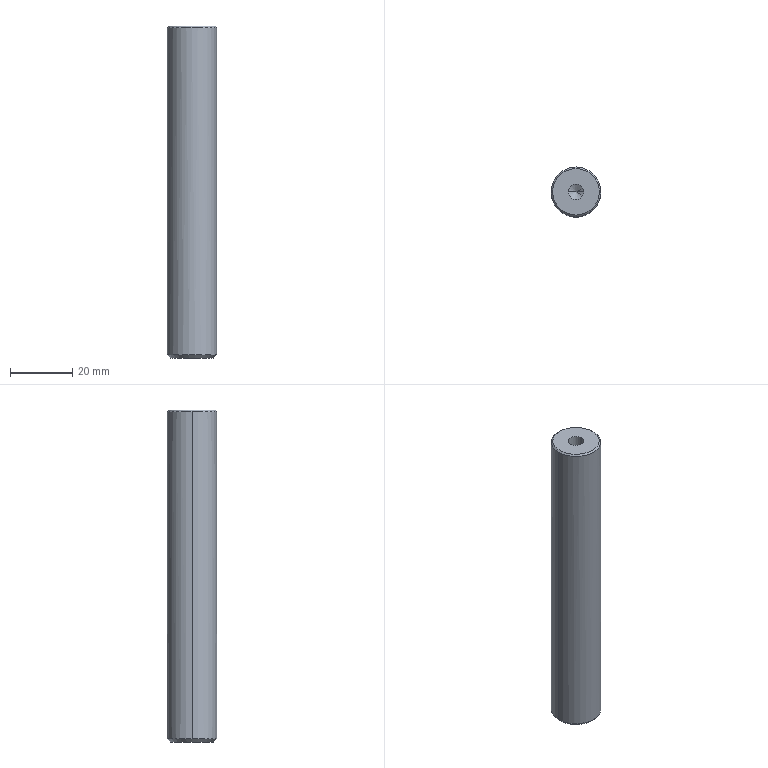Part | STEP file | PN_0006 Pre-compression sleeve guide rod | 1 solid | 16 faces | box 16 x 16 x 107 mm | volume 20796 mm3 | cone 8 | cylinder 6 | plane 2 | commonest cylinder face diameters 5 x4 16 x2
STEP:
#1=CARTESIAN_POINT('',(0.,0.,0.));
#2=DIRECTION('',(0.,0.,1.));
#3=DIRECTION('',(1.,0.,0.));
#4=AXIS2_PLACEMENT_3D('',#1,#2,#3);
#5=CARTESIAN_POINT('',(0.,8.,106.5));
#6=VERTEX_POINT('',#5);
#7=CARTESIAN_POINT('',(8.,0.,106.5));
#8=VERTEX_POINT('',#7);
#9=CARTESIAN_POINT('',(0.,0.,106.5));
#10=DIRECTION('',(0.,0.,-1.));
#11=DIRECTION('',(-1.,0.,0.));
#12=AXIS2_PLACEMENT_3D('',#9,#10,#11);
#13=CIRCLE('',#12,8.);
#14=CARTESIAN_POINT('',(0.,0.,107.));
#15=DIRECTION('',(0.,0.,-1.));
#16=DIRECTION('',(-1.,0.,0.));
#17=AXIS2_PLACEMENT_3D('',#14,#15,#16);
#18=CYLINDRICAL_SURFACE('',#17,8.);
#19=CARTESIAN_POINT('',(0.,0.5));
#20=DIRECTION('',(1.,0.));
#21=VECTOR('',#20,1.);
#22=LINE('',#19,#21);
#23=(GEOMETRIC_REPRESENTATION_CONTEXT(2)PARAMETRIC_REPRESENTATION_CONTEXT()REPRESENTATION_CONTEXT('',''));
#24=DEFINITIONAL_REPRESENTATION('',(#22),#23);
#25=PCURVE('',#18,#24);
#26=CARTESIAN_POINT('',(0.,0.,106.5));
#27=DIRECTION('',(0.,0.,-1.));
#28=DIRECTION('',(0.,1.,0.));
#29=AXIS2_PLACEMENT_3D('',#26,#27,#28);
#30=CONICAL_SURFACE('',#29,8.,0.7854);
#31=CARTESIAN_POINT('',(-1.571,0.));
#32=DIRECTION('',(1.,0.));
#33=VECTOR('',#32,1.);
#34=LINE('',#31,#33);
#35=(GEOMETRIC_REPRESENTATION_CONTEXT(2)PARAMETRIC_REPRESENTATION_CONTEXT()REPRESENTATION_CONTEXT('',''));
#36=DEFINITIONAL_REPRESENTATION('',(#34),#35);
#37=PCURVE('',#30,#36);
#38=SURFACE_CURVE('',#13,(#25,#37),.PCURVE_S1.);
#39=EDGE_CURVE('',#6,#8,#38,.T.);
#40=ORIENTED_EDGE('',*,*,#39,.T.);
#41=CARTESIAN_POINT('',(8.,0.,1.));
#42=VERTEX_POINT('',#41);
#43=CARTESIAN_POINT('',(8.,0.,107.));
#44=DIRECTION('',(0.,0.,-1.));
#45=VECTOR('',#44,1.);
#46=LINE('',#43,#45);
#47=CARTESIAN_POINT('',(3.142,0.));
#48=DIRECTION('',(0.,1.));
#49=VECTOR('',#48,1.);
#50=LINE('',#47,#49);
#51=(GEOMETRIC_REPRESENTATION_CONTEXT(2)PARAMETRIC_REPRESENTATION_CONTEXT()REPRESENTATION_CONTEXT('',''));
#52=DEFINITIONAL_REPRESENTATION('',(#50),#51);
#53=PCURVE('',#18,#52);
#54=CARTESIAN_POINT('',(0.,0.,107.));
#55=DIRECTION('',(0.,0.,-1.));
#56=DIRECTION('',(-1.,0.,0.));
#57=AXIS2_PLACEMENT_3D('',#54,#55,#56);
#58=CYLINDRICAL_SURFACE('',#57,8.);
#59=CARTESIAN_POINT('',(3.142,0.));
#60=DIRECTION('',(0.,1.));
#61=VECTOR('',#60,1.);
#62=LINE('',#59,#61);
#63=(GEOMETRIC_REPRESENTATION_CONTEXT(2)PARAMETRIC_REPRESENTATION_CONTEXT()REPRESENTATION_CONTEXT('',''));
#64=DEFINITIONAL_REPRESENTATION('',(#62),#63);
#65=PCURVE('',#58,#64);
#66=SURFACE_CURVE('',#46,(#53,#65),.PCURVE_S1.);
#67=EDGE_CURVE('',#8,#42,#66,.T.);
#68=ORIENTED_EDGE('',*,*,#67,.T.);
#69=CARTESIAN_POINT('',(-8.,0.,1.));
#70=VERTEX_POINT('',#69);
#71=CARTESIAN_POINT('',(0.,0.,1.));
#72=DIRECTION('',(0.,0.,1.));
#73=DIRECTION('',(-1.,0.,0.));
#74=AXIS2_PLACEMENT_3D('',#71,#72,#73);
#75=CIRCLE('',#74,8.);
#76=CARTESIAN_POINT('',(6.283,106.));
#77=DIRECTION('',(-1.,0.));
#78=VECTOR('',#77,1.);
#79=LINE('',#76,#78);
#80=(GEOMETRIC_REPRESENTATION_CONTEXT(2)PARAMETRIC_REPRESENTATION_CONTEXT()REPRESENTATION_CONTEXT('',''));
#81=DEFINITIONAL_REPRESENTATION('',(#79),#80);
#82=PCURVE('',#18,#81);
#83=CARTESIAN_POINT('',(0.,0.,1.));
#84=DIRECTION('',(0.,0.,1.));
#85=DIRECTION('',(1.,0.,0.));
#86=AXIS2_PLACEMENT_3D('',#83,#84,#85);
#87=CONICAL_SURFACE('',#86,8.,0.7854);
#88=CARTESIAN_POINT('',(-3.142,0.));
#89=DIRECTION('',(1.,0.));
#90=VECTOR('',#89,1.);
#91=LINE('',#88,#90);
#92=(GEOMETRIC_REPRESENTATION_CONTEXT(2)PARAMETRIC_REPRESENTATION_CONTEXT()REPRESENTATION_CONTEXT('',''));
#93=DEFINITIONAL_REPRESENTATION('',(#91),#92);
#94=PCURVE('',#87,#93);
#95=SURFACE_CURVE('',#75,(#82,#94),.PCURVE_S1.);
#96=EDGE_CURVE('',#42,#70,#95,.T.);
#97=ORIENTED_EDGE('',*,*,#96,.T.);
#98=CARTESIAN_POINT('',(-8.,0.,106.5));
#99=VERTEX_POINT('',#98);
#100=CARTESIAN_POINT('',(-8.,0.,107.));
#101=DIRECTION('',(0.,0.,-1.));
#102=VECTOR('',#101,1.);
#103=LINE('',#100,#102);
#104=CARTESIAN_POINT('',(0.,0.));
#105=DIRECTION('',(0.,1.));
#106=VECTOR('',#105,1.);
#107=LINE('',#104,#106);
#108=(GEOMETRIC_REPRESENTATION_CONTEXT(2)PARAMETRIC_REPRESENTATION_CONTEXT()REPRESENTATION_CONTEXT('',''));
#109=DEFINITIONAL_REPRESENTATION('',(#107),#108);
#110=PCURVE('',#18,#109);
#111=CARTESIAN_POINT('',(6.283,0.));
#112=DIRECTION('',(0.,1.));
#113=VECTOR('',#112,1.);
#114=LINE('',#111,#113);
#115=(GEOMETRIC_REPRESENTATION_CONTEXT(2)PARAMETRIC_REPRESENTATION_CONTEXT()REPRESENTATION_CONTEXT('',''));
#116=DEFINITIONAL_REPRESENTATION('',(#114),#115);
#117=PCURVE('',#58,#116);
#118=SURFACE_CURVE('',#103,(#110,#117),.PCURVE_S1.);
#119=EDGE_CURVE('',#99,#70,#118,.T.);
#120=ORIENTED_EDGE('',*,*,#119,.F.);
#121=CARTESIAN_POINT('',(0.,0.,106.5));
#122=DIRECTION('',(0.,0.,-1.));
#123=DIRECTION('',(-1.,0.,0.));
#124=AXIS2_PLACEMENT_3D('',#121,#122,#123);
#125=CIRCLE('',#124,8.);
#126=CARTESIAN_POINT('',(0.,0.5));
#127=DIRECTION('',(1.,0.));
#128=VECTOR('',#127,1.);
#129=LINE('',#126,#128);
#130=(GEOMETRIC_REPRESENTATION_CONTEXT(2)PARAMETRIC_REPRESENTATION_CONTEXT()REPRESENTATION_CONTEXT('',''));
#131=DEFINITIONAL_REPRESENTATION('',(#129),#130);
#132=PCURVE('',#18,#131);
#133=CARTESIAN_POINT('',(0.,0.,106.5));
#134=DIRECTION('',(0.,0.,-1.));
#135=DIRECTION('',(0.,1.,0.));
#136=AXIS2_PLACEMENT_3D('',#133,#134,#135);
#137=CONICAL_SURFACE('',#136,8.,0.7854);
#138=CARTESIAN_POINT('',(4.712,0.));
#139=DIRECTION('',(1.,0.));
#140=VECTOR('',#139,1.);
#141=LINE('',#138,#140);
#142=(GEOMETRIC_REPRESENTATION_CONTEXT(2)PARAMETRIC_REPRESENTATION_CONTEXT()REPRESENTATION_CONTEXT('',''));
#143=DEFINITIONAL_REPRESENTATION('',(#141),#142);
#144=PCURVE('',#137,#143);
#145=SURFACE_CURVE('',#125,(#132,#144),.PCURVE_S1.);
#146=EDGE_CURVE('',#99,#6,#145,.T.);
#147=ORIENTED_EDGE('',*,*,#146,.T.);
#148=EDGE_LOOP('',(#40,#68,#97,#120,#147));
#149=FACE_BOUND('',#148,.T.);
#150=ADVANCED_FACE('',(#149),#18,.T.);
#151=CARTESIAN_POINT('',(7.,0.,0.));
#152=VERTEX_POINT('',#151);
#153=CARTESIAN_POINT('',(-7.,0.,0.));
#154=VERTEX_POINT('',#153);
#155=CARTESIAN_POINT('',(0.,0.,0.));
#156=DIRECTION('',(0.,0.,1.));
#157=DIRECTION('',(1.,0.,0.));
#158=AXIS2_PLACEMENT_3D('',#155,#156,#157);
#159=CIRCLE('',#158,7.);
#160=CARTESIAN_POINT('',(0.,-1.));
#161=DIRECTION('',(1.,0.));
#162=VECTOR('',#161,1.);
#163=LINE('',#160,#162);
#164=(GEOMETRIC_REPRESENTATION_CONTEXT(2)PARAMETRIC_REPRESENTATION_CONTEXT()REPRESENTATION_CONTEXT('',''));
#165=DEFINITIONAL_REPRESENTATION('',(#163),#164);
#166=PCURVE('',#87,#165);
#167=CARTESIAN_POINT('',(0.,0.,0.));
#168=DIRECTION('',(0.,0.,1.));
#169=DIRECTION('',(1.,0.,0.));
#170=AXIS2_PLACEMENT_3D('',#167,#168,#169);
#171=PLANE('',#170);
#172=CARTESIAN_POINT('',(0.,0.));
#173=DIRECTION('',(1.,0.));
#174=AXIS2_PLACEMENT_2D('',#172,#173);
#175=CIRCLE('',#174,7.);
#176=(GEOMETRIC_REPRESENTATION_CONTEXT(2)PARAMETRIC_REPRESENTATION_CONTEXT()REPRESENTATION_CONTEXT('',''));
#177=DEFINITIONAL_REPRESENTATION('',(#175),#176);
#178=PCURVE('',#171,#177);
#179=SURFACE_CURVE('',#159,(#166,#178),.PCURVE_S1.);
#180=EDGE_CURVE('',#152,#154,#179,.T.);
#181=ORIENTED_EDGE('',*,*,#180,.T.);
#182=CARTESIAN_POINT('',(-8.,0.,1.));
#183=DIRECTION('',(-0.7071,0.,0.7071));
#184=VECTOR('',#183,1.);
#185=LINE('',#182,#184);
#186=CARTESIAN_POINT('',(3.142,0.));
#187=DIRECTION('',(0.,1.));
#188=VECTOR('',#187,1.);
#189=LINE('',#186,#188);
#190=(GEOMETRIC_REPRESENTATION_CONTEXT(2)PARAMETRIC_REPRESENTATION_CONTEXT()REPRESENTATION_CONTEXT('',''));
#191=DEFINITIONAL_REPRESENTATION('',(#189),#190);
#192=PCURVE('',#87,#191);
#193=CARTESIAN_POINT('',(0.,0.,1.));
#194=DIRECTION('',(0.,0.,1.));
#195=DIRECTION('',(1.,0.,0.));
#196=AXIS2_PLACEMENT_3D('',#193,#194,#195);
#197=CONICAL_SURFACE('',#196,8.,0.7854);
#198=CARTESIAN_POINT('',(3.142,0.));
#199=DIRECTION('',(0.,1.));
#200=VECTOR('',#199,1.);
#201=LINE('',#198,#200);
#202=(GEOMETRIC_REPRESENTATION_CONTEXT(2)PARAMETRIC_REPRESENTATION_CONTEXT()REPRESENTATION_CONTEXT('',''));
#203=DEFINITIONAL_REPRESENTATION('',(#201),#202);
#204=PCURVE('',#197,#203);
#205=SURFACE_CURVE('',#185,(#192,#204),.PCURVE_S1.);
#206=EDGE_CURVE('',#154,#70,#205,.T.);
#207=ORIENTED_EDGE('',*,*,#206,.T.);
#208=ORIENTED_EDGE('',*,*,#96,.F.);
#209=CARTESIAN_POINT('',(8.,0.,1.));
#210=DIRECTION('',(0.7071,0.,0.7071));
#211=VECTOR('',#210,1.);
#212=LINE('',#209,#211);
#213=CARTESIAN_POINT('',(0.,0.));
#214=DIRECTION('',(0.,1.));
#215=VECTOR('',#214,1.);
#216=LINE('',#213,#215);
#217=(GEOMETRIC_REPRESENTATION_CONTEXT(2)PARAMETRIC_REPRESENTATION_CONTEXT()REPRESENTATION_CONTEXT('',''));
#218=DEFINITIONAL_REPRESENTATION('',(#216),#217);
#219=PCURVE('',#87,#218);
#220=CARTESIAN_POINT('',(6.283,0.));
#221=DIRECTION('',(0.,1.));
#222=VECTOR('',#221,1.);
#223=LINE('',#220,#222);
#224=(GEOMETRIC_REPRESENTATION_CONTEXT(2)PARAMETRIC_REPRESENTATION_CONTEXT()REPRESENTATION_CONTEXT('',''));
#225=DEFINITIONAL_REPRESENTATION('',(#223),#224);
#226=PCURVE('',#197,#225);
#227=SURFACE_CURVE('',#212,(#219,#226),.PCURVE_S1.);
#228=EDGE_CURVE('',#152,#42,#227,.T.);
#229=ORIENTED_EDGE('',*,*,#228,.F.);
#230=EDGE_LOOP('',(#181,#207,#208,#229));
#231=FACE_BOUND('',#230,.T.);
#232=ADVANCED_FACE('',(#231),#87,.T.);
#233=CARTESIAN_POINT('',(0.,7.5,107.));
#234=VERTEX_POINT('',#233);
#235=CARTESIAN_POINT('',(0.,-7.5,107.));
#236=VERTEX_POINT('',#235);
#237=CARTESIAN_POINT('',(0.,0.,107.));
#238=DIRECTION('',(0.,0.,-1.));
#239=DIRECTION('',(0.,1.,0.));
#240=AXIS2_PLACEMENT_3D('',#237,#238,#239);
#241=CIRCLE('',#240,7.5);
#242=CARTESIAN_POINT('',(0.,-0.5));
#243=DIRECTION('',(1.,0.));
#244=VECTOR('',#243,1.);
#245=LINE('',#242,#244);
#246=(GEOMETRIC_REPRESENTATION_CONTEXT(2)PARAMETRIC_REPRESENTATION_CONTEXT()REPRESENTATION_CONTEXT('',''));
#247=DEFINITIONAL_REPRESENTATION('',(#245),#246);
#248=PCURVE('',#30,#247);
#249=CARTESIAN_POINT('',(0.,0.,107.));
#250=DIRECTION('',(0.,0.,1.));
#251=DIRECTION('',(1.,0.,0.));
#252=AXIS2_PLACEMENT_3D('',#249,#250,#251);
#253=PLANE('',#252);
#254=CARTESIAN_POINT('',(0.,7.5));
#255=CARTESIAN_POINT('',(12.99,7.5));
#256=CARTESIAN_POINT('',(6.495,-3.75));
#257=CARTESIAN_POINT('',(0.,-15.));
#258=CARTESIAN_POINT('',(-6.495,-3.75));
#259=CARTESIAN_POINT('',(-12.99,7.5));
#260=CARTESIAN_POINT('',(0.,7.5));
#261=(BOUNDED_CURVE()B_SPLINE_CURVE(2,(#254,#255,#256,#257,#258,#259,#260),.UNSPECIFIED.,.T.,.F.)B_SPLINE_CURVE_WITH_KNOTS((1,2,2,2,2,1),(-2.094,0.,2.094,4.189,6.283,8.378),.UNSPECIFIED.)CURVE()GEOMETRIC_REPRESENTATION_ITEM()RATIONAL_B_SPLINE_CURVE((1.,0.5,1.,0.5,1.,0.5,1.))REPRESENTATION_ITEM(''));
#262=(GEOMETRIC_REPRESENTATION_CONTEXT(2)PARAMETRIC_REPRESENTATION_CONTEXT()REPRESENTATION_CONTEXT('',''));
#263=DEFINITIONAL_REPRESENTATION('',(#261),#262);
#264=PCURVE('',#253,#263);
#265=SURFACE_CURVE('',#241,(#248,#264),.PCURVE_S1.);
#266=EDGE_CURVE('',#234,#236,#265,.T.);
#267=ORIENTED_EDGE('',*,*,#266,.T.);
#268=CARTESIAN_POINT('',(0.,-8.,106.5));
#269=VERTEX_POINT('',#268);
#270=CARTESIAN_POINT('',(0.,-8.,106.5));
#271=DIRECTION('',(0.,-0.7071,-0.7071));
#272=VECTOR('',#271,1.);
#273=LINE('',#270,#272);
#274=CARTESIAN_POINT('',(3.142,0.));
#275=DIRECTION('',(0.,1.));
#276=VECTOR('',#275,1.);
#277=LINE('',#274,#276);
#278=(GEOMETRIC_REPRESENTATION_CONTEXT(2)PARAMETRIC_REPRESENTATION_CONTEXT()REPRESENTATION_CONTEXT('',''));
#279=DEFINITIONAL_REPRESENTATION('',(#277),#278);
#280=PCURVE('',#30,#279);
#281=CARTESIAN_POINT('',(3.142,0.));
#282=DIRECTION('',(0.,1.));
#283=VECTOR('',#282,1.);
#284=LINE('',#281,#283);
#285=(GEOMETRIC_REPRESENTATION_CONTEXT(2)PARAMETRIC_REPRESENTATION_CONTEXT()REPRESENTATION_CONTEXT('',''));
#286=DEFINITIONAL_REPRESENTATION('',(#284),#285);
#287=PCURVE('',#137,#286);
#288=SURFACE_CURVE('',#273,(#280,#287),.PCURVE_S1.);
#289=EDGE_CURVE('',#236,#269,#288,.T.);
#290=ORIENTED_EDGE('',*,*,#289,.T.);
#291=CARTESIAN_POINT('',(0.,0.,106.5));
#292=DIRECTION('',(0.,0.,-1.));
#293=DIRECTION('',(-1.,0.,0.));
#294=AXIS2_PLACEMENT_3D('',#291,#292,#293);
#295=CIRCLE('',#294,8.);
#296=CARTESIAN_POINT('',(-1.571,0.));
#297=DIRECTION('',(1.,0.));
#298=VECTOR('',#297,1.);
#299=LINE('',#296,#298);
#300=(GEOMETRIC_REPRESENTATION_CONTEXT(2)PARAMETRIC_REPRESENTATION_CONTEXT()REPRESENTATION_CONTEXT('',''));
#301=DEFINITIONAL_REPRESENTATION('',(#299),#300);
#302=PCURVE('',#30,#301);
#303=CARTESIAN_POINT('',(0.,0.5));
#304=DIRECTION('',(1.,0.));
#305=VECTOR('',#304,1.);
#306=LINE('',#303,#305);
#307=(GEOMETRIC_REPRESENTATION_CONTEXT(2)PARAMETRIC_REPRESENTATION_CONTEXT()REPRESENTATION_CONTEXT('',''));
#308=DEFINITIONAL_REPRESENTATION('',(#306),#307);
#309=PCURVE('',#58,#308);
#310=SURFACE_CURVE('',#295,(#302,#309),.PCURVE_S1.);
#311=EDGE_CURVE('',#8,#269,#310,.T.);
#312=ORIENTED_EDGE('',*,*,#311,.F.);
#313=ORIENTED_EDGE('',*,*,#39,.F.);
#314=CARTESIAN_POINT('',(0.,8.,106.5));
#315=DIRECTION('',(0.,0.7071,-0.7071));
#316=VECTOR('',#315,1.);
#317=LINE('',#314,#316);
#318=CARTESIAN_POINT('',(0.,0.));
#319=DIRECTION('',(0.,1.));
#320=VECTOR('',#319,1.);
#321=LINE('',#318,#320);
#322=(GEOMETRIC_REPRESENTATION_CONTEXT(2)PARAMETRIC_REPRESENTATION_CONTEXT()REPRESENTATION_CONTEXT('',''));
#323=DEFINITIONAL_REPRESENTATION('',(#321),#322);
#324=PCURVE('',#30,#323);
#325=CARTESIAN_POINT('',(6.283,0.));
#326=DIRECTION('',(0.,1.));
#327=VECTOR('',#326,1.);
#328=LINE('',#325,#327);
#329=(GEOMETRIC_REPRESENTATION_CONTEXT(2)PARAMETRIC_REPRESENTATION_CONTEXT()REPRESENTATION_CONTEXT('',''));
#330=DEFINITIONAL_REPRESENTATION('',(#328),#329);
#331=PCURVE('',#137,#330);
#332=SURFACE_CURVE('',#317,(#324,#331),.PCURVE_S1.);
#333=EDGE_CURVE('',#234,#6,#332,.T.);
#334=ORIENTED_EDGE('',*,*,#333,.F.);
#335=EDGE_LOOP('',(#267,#290,#312,#313,#334));
#336=FACE_BOUND('',#335,.T.);
#337=ADVANCED_FACE('',(#336),#30,.T.);
#338=CARTESIAN_POINT('',(-2.5,0.,17.));
#339=VERTEX_POINT('',#338);
#340=CARTESIAN_POINT('',(-2.5,0.,0.));
#341=VERTEX_POINT('',#340);
#342=CARTESIAN_POINT('',(-2.5,0.,0.));
#343=DIRECTION('',(0.,0.,-1.));
#344=VECTOR('',#343,1.);
#345=LINE('',#342,#344);
#346=CARTESIAN_POINT('',(0.,0.,0.));
#347=DIRECTION('',(0.,0.,-1.));
#348=DIRECTION('',(-1.,0.,0.));
#349=AXIS2_PLACEMENT_3D('',#346,#347,#348);
#350=CYLINDRICAL_SURFACE('',#349,2.5);
#351=CARTESIAN_POINT('',(6.283,0.));
#352=DIRECTION('',(0.,1.));
#353=VECTOR('',#352,1.);
#354=LINE('',#351,#353);
#355=(GEOMETRIC_REPRESENTATION_CONTEXT(2)PARAMETRIC_REPRESENTATION_CONTEXT()REPRESENTATION_CONTEXT('',''));
#356=DEFINITIONAL_REPRESENTATION('',(#354),#355);
#357=PCURVE('',#350,#356);
#358=CARTESIAN_POINT('',(0.,0.,0.));
#359=DIRECTION('',(0.,0.,-1.));
#360=DIRECTION('',(-1.,0.,0.));
#361=AXIS2_PLACEMENT_3D('',#358,#359,#360);
#362=CYLINDRICAL_SURFACE('',#361,2.5);
#363=CARTESIAN_POINT('',(0.,0.));
#364=DIRECTION('',(0.,1.));
#365=VECTOR('',#364,1.);
#366=LINE('',#363,#365);
#367=(GEOMETRIC_REPRESENTATION_CONTEXT(2)PARAMETRIC_REPRESENTATION_CONTEXT()REPRESENTATION_CONTEXT('',''));
#368=DEFINITIONAL_REPRESENTATION('',(#366),#367);
#369=PCURVE('',#362,#368);
#370=SURFACE_CURVE('',#345,(#357,#369),.PCURVE_S1.);
#371=EDGE_CURVE('',#339,#341,#370,.T.);
#372=ORIENTED_EDGE('',*,*,#371,.T.);
#373=CARTESIAN_POINT('',(2.5,0.,0.));
#374=VERTEX_POINT('',#373);
#375=CARTESIAN_POINT('',(0.,0.,0.));
#376=DIRECTION('',(0.,0.,-1.));
#377=DIRECTION('',(-1.,0.,0.));
#378=AXIS2_PLACEMENT_3D('',#375,#376,#377);
#379=CIRCLE('',#378,2.5);
#380=CARTESIAN_POINT('',(0.,0.));
#381=DIRECTION('',(1.,0.));
#382=VECTOR('',#381,1.);
#383=LINE('',#380,#382);
#384=(GEOMETRIC_REPRESENTATION_CONTEXT(2)PARAMETRIC_REPRESENTATION_CONTEXT()REPRESENTATION_CONTEXT('',''));
#385=DEFINITIONAL_REPRESENTATION('',(#383),#384);
#386=PCURVE('',#350,#385);
#387=CARTESIAN_POINT('',(-2.5,0.));
#388=CARTESIAN_POINT('',(-2.5,4.33));
#389=CARTESIAN_POINT('',(1.25,2.165));
#390=CARTESIAN_POINT('',(5.,0.));
#391=CARTESIAN_POINT('',(1.25,-2.165));
#392=CARTESIAN_POINT('',(-2.5,-4.33));
#393=CARTESIAN_POINT('',(-2.5,0.));
#394=(BOUNDED_CURVE()B_SPLINE_CURVE(2,(#387,#388,#389,#390,#391,#392,#393),.UNSPECIFIED.,.T.,.F.)B_SPLINE_CURVE_WITH_KNOTS((1,2,2,2,2,1),(-2.094,0.,2.094,4.189,6.283,8.378),.UNSPECIFIED.)CURVE()GEOMETRIC_REPRESENTATION_ITEM()RATIONAL_B_SPLINE_CURVE((1.,0.5,1.,0.5,1.,0.5,1.))REPRESENTATION_ITEM(''));
#395=(GEOMETRIC_REPRESENTATION_CONTEXT(2)PARAMETRIC_REPRESENTATION_CONTEXT()REPRESENTATION_CONTEXT('',''));
#396=DEFINITIONAL_REPRESENTATION('',(#394),#395);
#397=PCURVE('',#171,#396);
#398=SURFACE_CURVE('',#379,(#386,#397),.PCURVE_S1.);
#399=EDGE_CURVE('',#374,#341,#398,.T.);
#400=ORIENTED_EDGE('',*,*,#399,.F.);
#401=CARTESIAN_POINT('',(2.5,0.,17.));
#402=VERTEX_POINT('',#401);
#403=CARTESIAN_POINT('',(2.5,0.,0.));
#404=DIRECTION('',(0.,0.,-1.));
#405=VECTOR('',#404,1.);
#406=LINE('',#403,#405);
#407=CARTESIAN_POINT('',(3.142,0.));
#408=DIRECTION('',(0.,1.));
#409=VECTOR('',#408,1.);
#410=LINE('',#407,#409);
#411=(GEOMETRIC_REPRESENTATION_CONTEXT(2)PARAMETRIC_REPRESENTATION_CONTEXT()REPRESENTATION_CONTEXT('',''));
#412=DEFINITIONAL_REPRESENTATION('',(#410),#411);
#413=PCURVE('',#350,#412);
#414=CARTESIAN_POINT('',(3.142,0.));
#415=DIRECTION('',(0.,1.));
#416=VECTOR('',#415,1.);
#417=LINE('',#414,#416);
#418=(GEOMETRIC_REPRESENTATION_CONTEXT(2)PARAMETRIC_REPRESENTATION_CONTEXT()REPRESENTATION_CONTEXT('',''));
#419=DEFINITIONAL_REPRESENTATION('',(#417),#418);
#420=PCURVE('',#362,#419);
#421=SURFACE_CURVE('',#406,(#413,#420),.PCURVE_S1.);
#422=EDGE_CURVE('',#402,#374,#421,.T.);
#423=ORIENTED_EDGE('',*,*,#422,.F.);
#424=CARTESIAN_POINT('',(0.,0.,17.));
#425=DIRECTION('',(0.,0.,-1.));
#426=DIRECTION('',(-1.,0.,0.));
#427=AXIS2_PLACEMENT_3D('',#424,#425,#426);
#428=CIRCLE('',#427,2.5);
#429=CARTESIAN_POINT('',(0.,-17.));
#430=DIRECTION('',(1.,0.));
#431=VECTOR('',#430,1.);
#432=LINE('',#429,#431);
#433=(GEOMETRIC_REPRESENTATION_CONTEXT(2)PARAMETRIC_REPRESENTATION_CONTEXT()REPRESENTATION_CONTEXT('',''));
#434=DEFINITIONAL_REPRESENTATION('',(#432),#433);
#435=PCURVE('',#350,#434);
#436=CARTESIAN_POINT('',(0.,0.,17.));
#437=DIRECTION('',(0.,0.,-1.));
#438=DIRECTION('',(-1.,0.,0.));
#439=AXIS2_PLACEMENT_3D('',#436,#437,#438);
#440=CONICAL_SURFACE('',#439,2.5,1.03);
#441=CARTESIAN_POINT('',(0.,0.));
#442=DIRECTION('',(1.,0.));
#443=VECTOR('',#442,1.);
#444=LINE('',#441,#443);
#445=(GEOMETRIC_REPRESENTATION_CONTEXT(2)PARAMETRIC_REPRESENTATION_CONTEXT()REPRESENTATION_CONTEXT('',''));
#446=DEFINITIONAL_REPRESENTATION('',(#444),#445);
#447=PCURVE('',#440,#446);
#448=SURFACE_CURVE('',#428,(#435,#447),.PCURVE_S1.);
#449=EDGE_CURVE('',#402,#339,#448,.T.);
#450=ORIENTED_EDGE('',*,*,#449,.T.);
#451=EDGE_LOOP('',(#372,#400,#423,#450));
#452=FACE_BOUND('',#451,.F.);
#453=ADVANCED_FACE('',(#452),#350,.F.);
#454=CARTESIAN_POINT('',(2.5,0.,90.));
#455=VERTEX_POINT('',#454);
#456=CARTESIAN_POINT('',(2.5,0.,107.));
#457=VERTEX_POINT('',#456);
#458=CARTESIAN_POINT('',(2.5,0.,107.));
#459=DIRECTION('',(0.,0.,1.));
#460=VECTOR('',#459,1.);
#461=LINE('',#458,#460);
#462=CARTESIAN_POINT('',(0.,0.,107.));
#463=DIRECTION('',(0.,0.,1.));
#464=DIRECTION('',(1.,0.,0.));
#465=AXIS2_PLACEMENT_3D('',#462,#463,#464);
#466=CYLINDRICAL_SURFACE('',#465,2.5);
#467=CARTESIAN_POINT('',(6.283,0.));
#468=DIRECTION('',(0.,1.));
#469=VECTOR('',#468,1.);
#470=LINE('',#467,#469);
#471=(GEOMETRIC_REPRESENTATION_CONTEXT(2)PARAMETRIC_REPRESENTATION_CONTEXT()REPRESENTATION_CONTEXT('',''));
#472=DEFINITIONAL_REPRESENTATION('',(#470),#471);
#473=PCURVE('',#466,#472);
#474=CARTESIAN_POINT('',(0.,0.,107.));
#475=DIRECTION('',(0.,0.,1.));
#476=DIRECTION('',(1.,0.,0.));
#477=AXIS2_PLACEMENT_3D('',#474,#475,#476);
#478=CYLINDRICAL_SURFACE('',#477,2.5);
#479=CARTESIAN_POINT('',(0.,0.));
#480=DIRECTION('',(0.,1.));
#481=VECTOR('',#480,1.);
#482=LINE('',#479,#481);
#483=(GEOMETRIC_REPRESENTATION_CONTEXT(2)PARAMETRIC_REPRESENTATION_CONTEXT()REPRESENTATION_CONTEXT('',''));
#484=DEFINITIONAL_REPRESENTATION('',(#482),#483);
#485=PCURVE('',#478,#484);
#486=SURFACE_CURVE('',#461,(#473,#485),.PCURVE_S1.);
#487=EDGE_CURVE('',#455,#457,#486,.T.);
#488=ORIENTED_EDGE('',*,*,#487,.T.);
#489=CARTESIAN_POINT('',(-2.5,0.,107.));
#490=VERTEX_POINT('',#489);
#491=CARTESIAN_POINT('',(0.,0.,107.));
#492=DIRECTION('',(0.,0.,-1.));
#493=DIRECTION('',(1.,0.,0.));
#494=AXIS2_PLACEMENT_3D('',#491,#492,#493);
#495=CIRCLE('',#494,2.5);
#496=CARTESIAN_POINT('',(6.283,0.));
#497=DIRECTION('',(-1.,0.));
#498=VECTOR('',#497,1.);
#499=LINE('',#496,#498);
#500=(GEOMETRIC_REPRESENTATION_CONTEXT(2)PARAMETRIC_REPRESENTATION_CONTEXT()REPRESENTATION_CONTEXT('',''));
#501=DEFINITIONAL_REPRESENTATION('',(#499),#500);
#502=PCURVE('',#466,#501);
#503=CARTESIAN_POINT('',(2.5,0.));
#504=CARTESIAN_POINT('',(2.5,-4.33));
#505=CARTESIAN_POINT('',(-1.25,-2.165));
#506=CARTESIAN_POINT('',(-5.,0.));
#507=CARTESIAN_POINT('',(-1.25,2.165));
#508=CARTESIAN_POINT('',(2.5,4.33));
#509=CARTESIAN_POINT('',(2.5,0.));
#510=(BOUNDED_CURVE()B_SPLINE_CURVE(2,(#503,#504,#505,#506,#507,#508,#509),.UNSPECIFIED.,.T.,.F.)B_SPLINE_CURVE_WITH_KNOTS((1,2,2,2,2,1),(-2.094,0.,2.094,4.189,6.283,8.378),.UNSPECIFIED.)CURVE()GEOMETRIC_REPRESENTATION_ITEM()RATIONAL_B_SPLINE_CURVE((1.,0.5,1.,0.5,1.,0.5,1.))REPRESENTATION_ITEM(''));
#511=(GEOMETRIC_REPRESENTATION_CONTEXT(2)PARAMETRIC_REPRESENTATION_CONTEXT()REPRESENTATION_CONTEXT('',''));
#512=DEFINITIONAL_REPRESENTATION('',(#510),#511);
#513=PCURVE('',#253,#512);
#514=SURFACE_CURVE('',#495,(#502,#513),.PCURVE_S1.);
#515=EDGE_CURVE('',#457,#490,#514,.T.);
#516=ORIENTED_EDGE('',*,*,#515,.T.);
#517=CARTESIAN_POINT('',(-2.5,0.,90.));
#518=VERTEX_POINT('',#517);
#519=CARTESIAN_POINT('',(-2.5,0.,107.));
#520=DIRECTION('',(0.,0.,1.));
#521=VECTOR('',#520,1.);
#522=LINE('',#519,#521);
#523=CARTESIAN_POINT('',(3.142,0.));
#524=DIRECTION('',(0.,1.));
#525=VECTOR('',#524,1.);
#526=LINE('',#523,#525);
#527=(GEOMETRIC_REPRESENTATION_CONTEXT(2)PARAMETRIC_REPRESENTATION_CONTEXT()REPRESENTATION_CONTEXT('',''));
#528=DEFINITIONAL_REPRESENTATION('',(#526),#527);
#529=PCURVE('',#466,#528);
#530=CARTESIAN_POINT('',(3.142,0.));
#531=DIRECTION('',(0.,1.));
#532=VECTOR('',#531,1.);
#533=LINE('',#530,#532);
#534=(GEOMETRIC_REPRESENTATION_CONTEXT(2)PARAMETRIC_REPRESENTATION_CONTEXT()REPRESENTATION_CONTEXT('',''));
#535=DEFINITIONAL_REPRESENTATION('',(#533),#534);
#536=PCURVE('',#478,#535);
#537=SURFACE_CURVE('',#522,(#529,#536),.PCURVE_S1.);
#538=EDGE_CURVE('',#518,#490,#537,.T.);
#539=ORIENTED_EDGE('',*,*,#538,.F.);
#540=CARTESIAN_POINT('',(0.,0.,90.));
#541=DIRECTION('',(0.,0.,1.));
#542=DIRECTION('',(1.,0.,0.));
#543=AXIS2_PLACEMENT_3D('',#540,#541,#542);
#544=CIRCLE('',#543,2.5);
#545=CARTESIAN_POINT('',(0.,-17.));
#546=DIRECTION('',(1.,0.));
#547=VECTOR('',#546,1.);
#548=LINE('',#545,#547);
#549=(GEOMETRIC_REPRESENTATION_CONTEXT(2)PARAMETRIC_REPRESENTATION_CONTEXT()REPRESENTATION_CONTEXT('',''));
#550=DEFINITIONAL_REPRESENTATION('',(#548),#549);
#551=PCURVE('',#466,#550);
#552=CARTESIAN_POINT('',(0.,0.,90.));
#553=DIRECTION('',(0.,0.,1.));
#554=DIRECTION('',(1.,0.,0.));
#555=AXIS2_PLACEMENT_3D('',#552,#553,#554);
#556=CONICAL_SURFACE('',#555,2.5,1.03);
#557=CARTESIAN_POINT('',(0.,0.));
#558=DIRECTION('',(1.,0.));
#559=VECTOR('',#558,1.);
#560=LINE('',#557,#559);
#561=(GEOMETRIC_REPRESENTATION_CONTEXT(2)PARAMETRIC_REPRESENTATION_CONTEXT()REPRESENTATION_CONTEXT('',''));
#562=DEFINITIONAL_REPRESENTATION('',(#560),#561);
#563=PCURVE('',#556,#562);
#564=SURFACE_CURVE('',#544,(#551,#563),.PCURVE_S1.);
#565=EDGE_CURVE('',#518,#455,#564,.T.);
#566=ORIENTED_EDGE('',*,*,#565,.T.);
#567=EDGE_LOOP('',(#488,#516,#539,#566));
#568=FACE_BOUND('',#567,.F.);
#569=ADVANCED_FACE('',(#568),#466,.F.);
#570=ORIENTED_EDGE('',*,*,#449,.F.);
#571=CARTESIAN_POINT('',(0.,0.,18.502));
#572=VERTEX_POINT('',#571);
#573=CARTESIAN_POINT('',(2.5,0.,17.));
#574=DIRECTION('',(0.8572,0.,-0.515));
#575=VECTOR('',#574,1.);
#576=LINE('',#573,#575);
#577=CARTESIAN_POINT('',(3.142,0.));
#578=DIRECTION('',(0.,1.));
#579=VECTOR('',#578,1.);
#580=LINE('',#577,#579);
#581=(GEOMETRIC_REPRESENTATION_CONTEXT(2)PARAMETRIC_REPRESENTATION_CONTEXT()REPRESENTATION_CONTEXT('',''));
#582=DEFINITIONAL_REPRESENTATION('',(#580),#581);
#583=PCURVE('',#440,#582);
#584=CARTESIAN_POINT('',(0.,0.,17.));
#585=DIRECTION('',(0.,0.,-1.));
#586=DIRECTION('',(-1.,0.,0.));
#587=AXIS2_PLACEMENT_3D('',#584,#585,#586);
#588=CONICAL_SURFACE('',#587,2.5,1.03);
#589=CARTESIAN_POINT('',(3.142,0.));
#590=DIRECTION('',(0.,1.));
#591=VECTOR('',#590,1.);
#592=LINE('',#589,#591);
#593=(GEOMETRIC_REPRESENTATION_CONTEXT(2)PARAMETRIC_REPRESENTATION_CONTEXT()REPRESENTATION_CONTEXT('',''));
#594=DEFINITIONAL_REPRESENTATION('',(#592),#593);
#595=PCURVE('',#588,#594);
#596=SURFACE_CURVE('',#576,(#583,#595),.PCURVE_S1.);
#597=EDGE_CURVE('',#572,#402,#596,.T.);
#598=ORIENTED_EDGE('',*,*,#597,.F.);
#599=CARTESIAN_POINT('',(-2.5,0.,17.));
#600=DIRECTION('',(-0.8572,0.,-0.515));
#601=VECTOR('',#600,1.);
#602=LINE('',#599,#601);
#603=CARTESIAN_POINT('',(6.283,0.));
#604=DIRECTION('',(0.,1.));
#605=VECTOR('',#604,1.);
#606=LINE('',#603,#605);
#607=(GEOMETRIC_REPRESENTATION_CONTEXT(2)PARAMETRIC_REPRESENTATION_CONTEXT()REPRESENTATION_CONTEXT('',''));
#608=DEFINITIONAL_REPRESENTATION('',(#606),#607);
#609=PCURVE('',#440,#608);
#610=CARTESIAN_POINT('',(0.,0.));
#611=DIRECTION('',(0.,1.));
#612=VECTOR('',#611,1.);
#613=LINE('',#610,#612);
#614=(GEOMETRIC_REPRESENTATION_CONTEXT(2)PARAMETRIC_REPRESENTATION_CONTEXT()REPRESENTATION_CONTEXT('',''));
#615=DEFINITIONAL_REPRESENTATION('',(#613),#614);
#616=PCURVE('',#588,#615);
#617=SURFACE_CURVE('',#602,(#609,#616),.PCURVE_S1.);
#618=EDGE_CURVE('',#572,#339,#617,.T.);
#619=ORIENTED_EDGE('',*,*,#618,.T.);
#620=EDGE_LOOP('',(#570,#598,#619));
#621=FACE_BOUND('',#620,.F.);
#622=ADVANCED_FACE('',(#621),#440,.F.);
#623=ORIENTED_EDGE('',*,*,#565,.F.);
#624=CARTESIAN_POINT('',(0.,0.,88.498));
#625=VERTEX_POINT('',#624);
#626=CARTESIAN_POINT('',(-2.5,0.,90.));
#627=DIRECTION('',(-0.8572,0.,0.515));
#628=VECTOR('',#627,1.);
#629=LINE('',#626,#628);
#630=CARTESIAN_POINT('',(3.142,0.));
#631=DIRECTION('',(0.,1.));
#632=VECTOR('',#631,1.);
#633=LINE('',#630,#632);
#634=(GEOMETRIC_REPRESENTATION_CONTEXT(2)PARAMETRIC_REPRESENTATION_CONTEXT()REPRESENTATION_CONTEXT('',''));
#635=DEFINITIONAL_REPRESENTATION('',(#633),#634);
#636=PCURVE('',#556,#635);
#637=CARTESIAN_POINT('',(0.,0.,90.));
#638=DIRECTION('',(0.,0.,1.));
#639=DIRECTION('',(1.,0.,0.));
#640=AXIS2_PLACEMENT_3D('',#637,#638,#639);
#641=CONICAL_SURFACE('',#640,2.5,1.03);
#642=CARTESIAN_POINT('',(3.142,0.));
#643=DIRECTION('',(0.,1.));
#644=VECTOR('',#643,1.);
#645=LINE('',#642,#644);
#646=(GEOMETRIC_REPRESENTATION_CONTEXT(2)PARAMETRIC_REPRESENTATION_CONTEXT()REPRESENTATION_CONTEXT('',''));
#647=DEFINITIONAL_REPRESENTATION('',(#645),#646);
#648=PCURVE('',#641,#647);
#649=SURFACE_CURVE('',#629,(#636,#648),.PCURVE_S1.);
#650=EDGE_CURVE('',#625,#518,#649,.T.);
#651=ORIENTED_EDGE('',*,*,#650,.F.);
#652=CARTESIAN_POINT('',(2.5,0.,90.));
#653=DIRECTION('',(0.8572,0.,0.515));
#654=VECTOR('',#653,1.);
#655=LINE('',#652,#654);
#656=CARTESIAN_POINT('',(6.283,0.));
#657=DIRECTION('',(0.,1.));
#658=VECTOR('',#657,1.);
#659=LINE('',#656,#658);
#660=(GEOMETRIC_REPRESENTATION_CONTEXT(2)PARAMETRIC_REPRESENTATION_CONTEXT()REPRESENTATION_CONTEXT('',''));
#661=DEFINITIONAL_REPRESENTATION('',(#659),#660);
#662=PCURVE('',#556,#661);
#663=CARTESIAN_POINT('',(0.,0.));
#664=DIRECTION('',(0.,1.));
#665=VECTOR('',#664,1.);
#666=LINE('',#663,#665);
#667=(GEOMETRIC_REPRESENTATION_CONTEXT(2)PARAMETRIC_REPRESENTATION_CONTEXT()REPRESENTATION_CONTEXT('',''));
#668=DEFINITIONAL_REPRESENTATION('',(#666),#667);
#669=PCURVE('',#641,#668);
#670=SURFACE_CURVE('',#655,(#662,#669),.PCURVE_S1.);
#671=EDGE_CURVE('',#625,#455,#670,.T.);
#672=ORIENTED_EDGE('',*,*,#671,.T.);
#673=EDGE_LOOP('',(#623,#651,#672));
#674=FACE_BOUND('',#673,.F.);
#675=ADVANCED_FACE('',(#674),#556,.F.);
#676=ORIENTED_EDGE('',*,*,#67,.F.);
#677=ORIENTED_EDGE('',*,*,#311,.T.);
#678=CARTESIAN_POINT('',(0.,0.,106.5));
#679=DIRECTION('',(0.,0.,-1.));
#680=DIRECTION('',(-1.,0.,0.));
#681=AXIS2_PLACEMENT_3D('',#678,#679,#680);
#682=CIRCLE('',#681,8.);
#683=CARTESIAN_POINT('',(0.,0.5));
#684=DIRECTION('',(1.,0.));
#685=VECTOR('',#684,1.);
#686=LINE('',#683,#685);
#687=(GEOMETRIC_REPRESENTATION_CONTEXT(2)PARAMETRIC_REPRESENTATION_CONTEXT()REPRESENTATION_CONTEXT('',''));
#688=DEFINITIONAL_REPRESENTATION('',(#686),#687);
#689=PCURVE('',#58,#688);
#690=CARTESIAN_POINT('',(-1.571,0.));
#691=DIRECTION('',(1.,0.));
#692=VECTOR('',#691,1.);
#693=LINE('',#690,#692);
#694=(GEOMETRIC_REPRESENTATION_CONTEXT(2)PARAMETRIC_REPRESENTATION_CONTEXT()REPRESENTATION_CONTEXT('',''));
#695=DEFINITIONAL_REPRESENTATION('',(#693),#694);
#696=PCURVE('',#137,#695);
#697=SURFACE_CURVE('',#682,(#689,#696),.PCURVE_S1.);
#698=EDGE_CURVE('',#269,#99,#697,.T.);
#699=ORIENTED_EDGE('',*,*,#698,.T.);
#700=ORIENTED_EDGE('',*,*,#119,.T.);
#701=CARTESIAN_POINT('',(0.,0.,1.));
#702=DIRECTION('',(0.,0.,1.));
#703=DIRECTION('',(-1.,0.,0.));
#704=AXIS2_PLACEMENT_3D('',#701,#702,#703);
#705=CIRCLE('',#704,8.);
#706=CARTESIAN_POINT('',(6.283,106.));
#707=DIRECTION('',(-1.,0.));
#708=VECTOR('',#707,1.);
#709=LINE('',#706,#708);
#710=(GEOMETRIC_REPRESENTATION_CONTEXT(2)PARAMETRIC_REPRESENTATION_CONTEXT()REPRESENTATION_CONTEXT('',''));
#711=DEFINITIONAL_REPRESENTATION('',(#709),#710);
#712=PCURVE('',#58,#711);
#713=CARTESIAN_POINT('',(3.142,0.));
#714=DIRECTION('',(1.,0.));
#715=VECTOR('',#714,1.);
#716=LINE('',#713,#715);
#717=(GEOMETRIC_REPRESENTATION_CONTEXT(2)PARAMETRIC_REPRESENTATION_CONTEXT()REPRESENTATION_CONTEXT('',''));
#718=DEFINITIONAL_REPRESENTATION('',(#716),#717);
#719=PCURVE('',#197,#718);
#720=SURFACE_CURVE('',#705,(#712,#719),.PCURVE_S1.);
#721=EDGE_CURVE('',#70,#42,#720,.T.);
#722=ORIENTED_EDGE('',*,*,#721,.T.);
#723=EDGE_LOOP('',(#676,#677,#699,#700,#722));
#724=FACE_BOUND('',#723,.T.);
#725=ADVANCED_FACE('',(#724),#58,.T.);
#726=ORIENTED_EDGE('',*,*,#206,.F.);
#727=CARTESIAN_POINT('',(0.,0.,0.));
#728=DIRECTION('',(0.,0.,1.));
#729=DIRECTION('',(1.,0.,0.));
#730=AXIS2_PLACEMENT_3D('',#727,#728,#729);
#731=CIRCLE('',#730,7.);
#732=CARTESIAN_POINT('',(0.,-1.));
#733=DIRECTION('',(1.,0.));
#734=VECTOR('',#733,1.);
#735=LINE('',#732,#734);
#736=(GEOMETRIC_REPRESENTATION_CONTEXT(2)PARAMETRIC_REPRESENTATION_CONTEXT()REPRESENTATION_CONTEXT('',''));
#737=DEFINITIONAL_REPRESENTATION('',(#735),#736);
#738=PCURVE('',#197,#737);
#739=CARTESIAN_POINT('',(0.,0.));
#740=DIRECTION('',(1.,0.));
#741=AXIS2_PLACEMENT_2D('',#739,#740);
#742=CIRCLE('',#741,7.);
#743=(GEOMETRIC_REPRESENTATION_CONTEXT(2)PARAMETRIC_REPRESENTATION_CONTEXT()REPRESENTATION_CONTEXT('',''));
#744=DEFINITIONAL_REPRESENTATION('',(#742),#743);
#745=PCURVE('',#171,#744);
#746=SURFACE_CURVE('',#731,(#738,#745),.PCURVE_S1.);
#747=EDGE_CURVE('',#154,#152,#746,.T.);
#748=ORIENTED_EDGE('',*,*,#747,.T.);
#749=ORIENTED_EDGE('',*,*,#228,.T.);
#750=ORIENTED_EDGE('',*,*,#721,.F.);
#751=EDGE_LOOP('',(#726,#748,#749,#750));
#752=FACE_BOUND('',#751,.T.);
#753=ADVANCED_FACE('',(#752),#197,.T.);
#754=ORIENTED_EDGE('',*,*,#289,.F.);
#755=CARTESIAN_POINT('',(0.,0.,107.));
#756=DIRECTION('',(0.,0.,-1.));
#757=DIRECTION('',(0.,1.,0.));
#758=AXIS2_PLACEMENT_3D('',#755,#756,#757);
#759=CIRCLE('',#758,7.5);
#760=CARTESIAN_POINT('',(0.,-0.5));
#761=DIRECTION('',(1.,0.));
#762=VECTOR('',#761,1.);
#763=LINE('',#760,#762);
#764=(GEOMETRIC_REPRESENTATION_CONTEXT(2)PARAMETRIC_REPRESENTATION_CONTEXT()REPRESENTATION_CONTEXT('',''));
#765=DEFINITIONAL_REPRESENTATION('',(#763),#764);
#766=PCURVE('',#137,#765);
#767=CARTESIAN_POINT('',(0.,7.5));
#768=CARTESIAN_POINT('',(12.99,7.5));
#769=CARTESIAN_POINT('',(6.495,-3.75));
#770=CARTESIAN_POINT('',(0.,-15.));
#771=CARTESIAN_POINT('',(-6.495,-3.75));
#772=CARTESIAN_POINT('',(-12.99,7.5));
#773=CARTESIAN_POINT('',(0.,7.5));
#774=(BOUNDED_CURVE()B_SPLINE_CURVE(2,(#767,#768,#769,#770,#771,#772,#773),.UNSPECIFIED.,.T.,.F.)B_SPLINE_CURVE_WITH_KNOTS((1,2,2,2,2,1),(-2.094,0.,2.094,4.189,6.283,8.378),.UNSPECIFIED.)CURVE()GEOMETRIC_REPRESENTATION_ITEM()RATIONAL_B_SPLINE_CURVE((1.,0.5,1.,0.5,1.,0.5,1.))REPRESENTATION_ITEM(''));
#775=(GEOMETRIC_REPRESENTATION_CONTEXT(2)PARAMETRIC_REPRESENTATION_CONTEXT()REPRESENTATION_CONTEXT('',''));
#776=DEFINITIONAL_REPRESENTATION('',(#774),#775);
#777=PCURVE('',#253,#776);
#778=SURFACE_CURVE('',#759,(#766,#777),.PCURVE_S1.);
#779=EDGE_CURVE('',#236,#234,#778,.T.);
#780=ORIENTED_EDGE('',*,*,#779,.T.);
#781=ORIENTED_EDGE('',*,*,#333,.T.);
#782=ORIENTED_EDGE('',*,*,#146,.F.);
#783=ORIENTED_EDGE('',*,*,#698,.F.);
#784=EDGE_LOOP('',(#754,#780,#781,#782,#783));
#785=FACE_BOUND('',#784,.T.);
#786=ADVANCED_FACE('',(#785),#137,.T.);
#787=ORIENTED_EDGE('',*,*,#180,.F.);
#788=ORIENTED_EDGE('',*,*,#747,.F.);
#789=EDGE_LOOP('',(#787,#788));
#790=FACE_BOUND('',#789,.T.);
#791=CARTESIAN_POINT('',(0.,0.,0.));
#792=DIRECTION('',(0.,0.,-1.));
#793=DIRECTION('',(-1.,0.,0.));
#794=AXIS2_PLACEMENT_3D('',#791,#792,#793);
#795=CIRCLE('',#794,2.5);
#796=CARTESIAN_POINT('',(-2.5,0.));
#797=CARTESIAN_POINT('',(-2.5,4.33));
#798=CARTESIAN_POINT('',(1.25,2.165));
#799=CARTESIAN_POINT('',(5.,0.));
#800=CARTESIAN_POINT('',(1.25,-2.165));
#801=CARTESIAN_POINT('',(-2.5,-4.33));
#802=CARTESIAN_POINT('',(-2.5,0.));
#803=(BOUNDED_CURVE()B_SPLINE_CURVE(2,(#796,#797,#798,#799,#800,#801,#802),.UNSPECIFIED.,.T.,.F.)B_SPLINE_CURVE_WITH_KNOTS((1,2,2,2,2,1),(-2.094,0.,2.094,4.189,6.283,8.378),.UNSPECIFIED.)CURVE()GEOMETRIC_REPRESENTATION_ITEM()RATIONAL_B_SPLINE_CURVE((1.,0.5,1.,0.5,1.,0.5,1.))REPRESENTATION_ITEM(''));
#804=(GEOMETRIC_REPRESENTATION_CONTEXT(2)PARAMETRIC_REPRESENTATION_CONTEXT()REPRESENTATION_CONTEXT('',''));
#805=DEFINITIONAL_REPRESENTATION('',(#803),#804);
#806=PCURVE('',#171,#805);
#807=CARTESIAN_POINT('',(0.,0.));
#808=DIRECTION('',(1.,0.));
#809=VECTOR('',#808,1.);
#810=LINE('',#807,#809);
#811=(GEOMETRIC_REPRESENTATION_CONTEXT(2)PARAMETRIC_REPRESENTATION_CONTEXT()REPRESENTATION_CONTEXT('',''));
#812=DEFINITIONAL_REPRESENTATION('',(#810),#811);
#813=PCURVE('',#362,#812);
#814=SURFACE_CURVE('',#795,(#806,#813),.PCURVE_S1.);
#815=EDGE_CURVE('',#341,#374,#814,.T.);
#816=ORIENTED_EDGE('',*,*,#815,.F.);
#817=ORIENTED_EDGE('',*,*,#399,.F.);
#818=EDGE_LOOP('',(#816,#817));
#819=FACE_BOUND('',#818,.T.);
#820=ADVANCED_FACE('',(#790,#819),#171,.F.);
#821=ORIENTED_EDGE('',*,*,#266,.F.);
#822=ORIENTED_EDGE('',*,*,#779,.F.);
#823=EDGE_LOOP('',(#821,#822));
#824=FACE_BOUND('',#823,.T.);
#825=ORIENTED_EDGE('',*,*,#515,.T.);
#826=CARTESIAN_POINT('',(0.,0.,107.));
#827=DIRECTION('',(0.,0.,-1.));
#828=DIRECTION('',(1.,0.,0.));
#829=AXIS2_PLACEMENT_3D('',#826,#827,#828);
#830=CIRCLE('',#829,2.5);
#831=CARTESIAN_POINT('',(2.5,0.));
#832=CARTESIAN_POINT('',(2.5,-4.33));
#833=CARTESIAN_POINT('',(-1.25,-2.165));
#834=CARTESIAN_POINT('',(-5.,0.));
#835=CARTESIAN_POINT('',(-1.25,2.165));
#836=CARTESIAN_POINT('',(2.5,4.33));
#837=CARTESIAN_POINT('',(2.5,0.));
#838=(BOUNDED_CURVE()B_SPLINE_CURVE(2,(#831,#832,#833,#834,#835,#836,#837),.UNSPECIFIED.,.T.,.F.)B_SPLINE_CURVE_WITH_KNOTS((1,2,2,2,2,1),(-2.094,0.,2.094,4.189,6.283,8.378),.UNSPECIFIED.)CURVE()GEOMETRIC_REPRESENTATION_ITEM()RATIONAL_B_SPLINE_CURVE((1.,0.5,1.,0.5,1.,0.5,1.))REPRESENTATION_ITEM(''));
#839=(GEOMETRIC_REPRESENTATION_CONTEXT(2)PARAMETRIC_REPRESENTATION_CONTEXT()REPRESENTATION_CONTEXT('',''));
#840=DEFINITIONAL_REPRESENTATION('',(#838),#839);
#841=PCURVE('',#253,#840);
#842=CARTESIAN_POINT('',(6.283,0.));
#843=DIRECTION('',(-1.,0.));
#844=VECTOR('',#843,1.);
#845=LINE('',#842,#844);
#846=(GEOMETRIC_REPRESENTATION_CONTEXT(2)PARAMETRIC_REPRESENTATION_CONTEXT()REPRESENTATION_CONTEXT('',''));
#847=DEFINITIONAL_REPRESENTATION('',(#845),#846);
#848=PCURVE('',#478,#847);
#849=SURFACE_CURVE('',#830,(#841,#848),.PCURVE_S1.);
#850=EDGE_CURVE('',#490,#457,#849,.T.);
#851=ORIENTED_EDGE('',*,*,#850,.T.);
#852=EDGE_LOOP('',(#825,#851));
#853=FACE_BOUND('',#852,.T.);
#854=ADVANCED_FACE('',(#824,#853),#253,.T.);
#855=ORIENTED_EDGE('',*,*,#815,.F.);
#856=ORIENTED_EDGE('',*,*,#371,.F.);
#857=CARTESIAN_POINT('',(0.,0.,17.));
#858=DIRECTION('',(0.,0.,-1.));
#859=DIRECTION('',(-1.,0.,0.));
#860=AXIS2_PLACEMENT_3D('',#857,#858,#859);
#861=CIRCLE('',#860,2.5);
#862=CARTESIAN_POINT('',(0.,-17.));
#863=DIRECTION('',(1.,0.));
#864=VECTOR('',#863,1.);
#865=LINE('',#862,#864);
#866=(GEOMETRIC_REPRESENTATION_CONTEXT(2)PARAMETRIC_REPRESENTATION_CONTEXT()REPRESENTATION_CONTEXT('',''));
#867=DEFINITIONAL_REPRESENTATION('',(#865),#866);
#868=PCURVE('',#362,#867);
#869=CARTESIAN_POINT('',(0.,0.));
#870=DIRECTION('',(1.,0.));
#871=VECTOR('',#870,1.);
#872=LINE('',#869,#871);
#873=(GEOMETRIC_REPRESENTATION_CONTEXT(2)PARAMETRIC_REPRESENTATION_CONTEXT()REPRESENTATION_CONTEXT('',''));
#874=DEFINITIONAL_REPRESENTATION('',(#872),#873);
#875=PCURVE('',#588,#874);
#876=SURFACE_CURVE('',#861,(#868,#875),.PCURVE_S1.);
#877=EDGE_CURVE('',#339,#402,#876,.T.);
#878=ORIENTED_EDGE('',*,*,#877,.T.);
#879=ORIENTED_EDGE('',*,*,#422,.T.);
#880=EDGE_LOOP('',(#855,#856,#878,#879));
#881=FACE_BOUND('',#880,.F.);
#882=ADVANCED_FACE('',(#881),#362,.F.);
#883=ORIENTED_EDGE('',*,*,#850,.T.);
#884=ORIENTED_EDGE('',*,*,#487,.F.);
#885=CARTESIAN_POINT('',(0.,0.,90.));
#886=DIRECTION('',(0.,0.,1.));
#887=DIRECTION('',(1.,0.,0.));
#888=AXIS2_PLACEMENT_3D('',#885,#886,#887);
#889=CIRCLE('',#888,2.5);
#890=CARTESIAN_POINT('',(0.,-17.));
#891=DIRECTION('',(1.,0.));
#892=VECTOR('',#891,1.);
#893=LINE('',#890,#892);
#894=(GEOMETRIC_REPRESENTATION_CONTEXT(2)PARAMETRIC_REPRESENTATION_CONTEXT()REPRESENTATION_CONTEXT('',''));
#895=DEFINITIONAL_REPRESENTATION('',(#893),#894);
#896=PCURVE('',#478,#895);
#897=CARTESIAN_POINT('',(0.,0.));
#898=DIRECTION('',(1.,0.));
#899=VECTOR('',#898,1.);
#900=LINE('',#897,#899);
#901=(GEOMETRIC_REPRESENTATION_CONTEXT(2)PARAMETRIC_REPRESENTATION_CONTEXT()REPRESENTATION_CONTEXT('',''));
#902=DEFINITIONAL_REPRESENTATION('',(#900),#901);
#903=PCURVE('',#641,#902);
#904=SURFACE_CURVE('',#889,(#896,#903),.PCURVE_S1.);
#905=EDGE_CURVE('',#455,#518,#904,.T.);
#906=ORIENTED_EDGE('',*,*,#905,.T.);
#907=ORIENTED_EDGE('',*,*,#538,.T.);
#908=EDGE_LOOP('',(#883,#884,#906,#907));
#909=FACE_BOUND('',#908,.F.);
#910=ADVANCED_FACE('',(#909),#478,.F.);
#911=ORIENTED_EDGE('',*,*,#877,.F.);
#912=ORIENTED_EDGE('',*,*,#618,.F.);
#913=ORIENTED_EDGE('',*,*,#597,.T.);
#914=EDGE_LOOP('',(#911,#912,#913));
#915=FACE_BOUND('',#914,.F.);
#916=ADVANCED_FACE('',(#915),#588,.F.);
#917=ORIENTED_EDGE('',*,*,#905,.F.);
#918=ORIENTED_EDGE('',*,*,#671,.F.);
#919=ORIENTED_EDGE('',*,*,#650,.T.);
#920=EDGE_LOOP('',(#917,#918,#919));
#921=FACE_BOUND('',#920,.F.);
#922=ADVANCED_FACE('',(#921),#641,.F.);
#923=CLOSED_SHELL('',(#150,#232,#337,#453,#569,#622,#675,#725,#753,#786,#820,#854,#882,#910,#916,#922));
#924=MANIFOLD_SOLID_BREP('',#923);
#925=(LENGTH_UNIT()NAMED_UNIT(*)SI_UNIT(.MILLI.,.METRE.));
#926=UNCERTAINTY_MEASURE_WITH_UNIT(LENGTH_MEASURE(0.0000001),#925,'','');
#927=(NAMED_UNIT(*)PLANE_ANGLE_UNIT()SI_UNIT($,.RADIAN.));
#928=(NAMED_UNIT(*)SI_UNIT($,.STERADIAN.)SOLID_ANGLE_UNIT());
#929=(GEOMETRIC_REPRESENTATION_CONTEXT(3)GLOBAL_UNCERTAINTY_ASSIGNED_CONTEXT((#926))GLOBAL_UNIT_ASSIGNED_CONTEXT((#925,#927,#928))REPRESENTATION_CONTEXT('',''));
#930=ADVANCED_BREP_SHAPE_REPRESENTATION('',(#4,#924),#929);